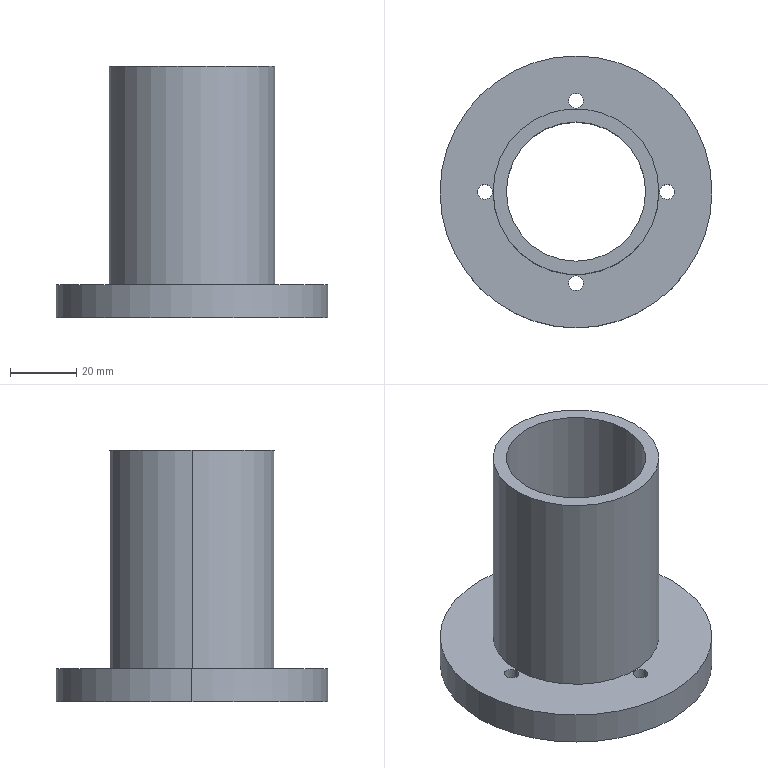Part | SolidWorks | features 3DProfileFeature 1, CirPattern 1, Extrusion 1, HoleWzd 1, ICE 1 | 1 solid | 29 faces | box 82 x 82 x 76 mm | volume 75839 mm3 | cylinder 22 | plane 7 | commonest cylinder face diameters 4.5 x8 8 x8 42 x2 50 x2 82 x2
STEP:
#1=CARTESIAN_POINT('',(31.5,0.,-5.4));
#2=VERTEX_POINT('',#1);
#3=CARTESIAN_POINT('',(23.5,0.,-5.4));
#4=VERTEX_POINT('',#3);
#5=CARTESIAN_POINT('',(27.5,0.,-5.4));
#6=DIRECTION('',(0.,0.,-1.));
#7=DIRECTION('',(-1.,0.,0.));
#8=AXIS2_PLACEMENT_3D('',#5,#6,#7);
#9=CIRCLE('',#8,4.);
#10=EDGE_CURVE('',#2,#4,#9,.T.);
#11=ORIENTED_EDGE('',*,*,#10,.F.);
#12=CARTESIAN_POINT('',(31.5,0.,-10.));
#13=VERTEX_POINT('',#12);
#14=CARTESIAN_POINT('',(31.5,0.,-10.));
#15=DIRECTION('',(0.,0.,-1.));
#16=VECTOR('',#15,1000.);
#17=LINE('',#14,#16);
#18=EDGE_CURVE('',#2,#13,#17,.T.);
#19=ORIENTED_EDGE('',*,*,#18,.T.);
#20=CARTESIAN_POINT('',(23.5,0.,-10.));
#21=VERTEX_POINT('',#20);
#22=CARTESIAN_POINT('',(27.5,0.,-10.));
#23=DIRECTION('',(0.,0.,-1.));
#24=DIRECTION('',(-1.,0.,0.));
#25=AXIS2_PLACEMENT_3D('',#22,#23,#24);
#26=CIRCLE('',#25,4.);
#27=EDGE_CURVE('',#13,#21,#26,.T.);
#28=ORIENTED_EDGE('',*,*,#27,.T.);
#29=CARTESIAN_POINT('',(23.5,0.,-10.));
#30=DIRECTION('',(0.,0.,-1.));
#31=VECTOR('',#30,1000.);
#32=LINE('',#29,#31);
#33=EDGE_CURVE('',#4,#21,#32,.T.);
#34=ORIENTED_EDGE('',*,*,#33,.F.);
#35=EDGE_LOOP('',(#11,#19,#28,#34));
#36=FACE_OUTER_BOUND('',#35,.T.);
#37=CARTESIAN_POINT('',(27.5,0.,-10.));
#38=DIRECTION('',(0.,0.,-1.));
#39=DIRECTION('',(-1.,0.,0.));
#40=AXIS2_PLACEMENT_3D('',#37,#38,#39);
#41=CYLINDRICAL_SURFACE('',#40,4.);
#42=ADVANCED_FACE('',(#36),#41,.F.);
#43=CARTESIAN_POINT('',(29.75,0.,0.));
#44=VERTEX_POINT('',#43);
#45=CARTESIAN_POINT('',(25.25,0.,0.));
#46=VERTEX_POINT('',#45);
#47=CARTESIAN_POINT('',(27.5,0.,0.));
#48=DIRECTION('',(0.,0.,-1.));
#49=DIRECTION('',(-1.,0.,0.));
#50=AXIS2_PLACEMENT_3D('',#47,#48,#49);
#51=CIRCLE('',#50,2.25);
#52=EDGE_CURVE('',#44,#46,#51,.T.);
#53=ORIENTED_EDGE('',*,*,#52,.F.);
#54=CARTESIAN_POINT('',(29.75,0.,-5.4));
#55=VERTEX_POINT('',#54);
#56=CARTESIAN_POINT('',(29.75,0.,-10.));
#57=DIRECTION('',(0.,0.,-1.));
#58=VECTOR('',#57,1000.);
#59=LINE('',#56,#58);
#60=EDGE_CURVE('',#44,#55,#59,.T.);
#61=ORIENTED_EDGE('',*,*,#60,.T.);
#62=CARTESIAN_POINT('',(25.25,0.,-5.4));
#63=VERTEX_POINT('',#62);
#64=CARTESIAN_POINT('',(27.5,0.,-5.4));
#65=DIRECTION('',(0.,0.,-1.));
#66=DIRECTION('',(-1.,0.,0.));
#67=AXIS2_PLACEMENT_3D('',#64,#65,#66);
#68=CIRCLE('',#67,2.25);
#69=EDGE_CURVE('',#55,#63,#68,.T.);
#70=ORIENTED_EDGE('',*,*,#69,.T.);
#71=CARTESIAN_POINT('',(25.25,0.,-10.));
#72=DIRECTION('',(0.,0.,-1.));
#73=VECTOR('',#72,1000.);
#74=LINE('',#71,#73);
#75=EDGE_CURVE('',#46,#63,#74,.T.);
#76=ORIENTED_EDGE('',*,*,#75,.F.);
#77=EDGE_LOOP('',(#53,#61,#70,#76));
#78=FACE_OUTER_BOUND('',#77,.T.);
#79=CARTESIAN_POINT('',(27.5,0.,-10.));
#80=DIRECTION('',(0.,0.,-1.));
#81=DIRECTION('',(-1.,0.,0.));
#82=AXIS2_PLACEMENT_3D('',#79,#80,#81);
#83=CYLINDRICAL_SURFACE('',#82,2.25);
#84=ADVANCED_FACE('',(#78),#83,.F.);
#85=CARTESIAN_POINT('',(4.,27.5,-5.4));
#86=VERTEX_POINT('',#85);
#87=CARTESIAN_POINT('',(-4.,27.5,-5.4));
#88=VERTEX_POINT('',#87);
#89=CARTESIAN_POINT('',(0.,27.5,-5.4));
#90=DIRECTION('',(0.,0.,-1.));
#91=DIRECTION('',(-1.,0.,0.));
#92=AXIS2_PLACEMENT_3D('',#89,#90,#91);
#93=CIRCLE('',#92,4.);
#94=EDGE_CURVE('',#86,#88,#93,.T.);
#95=ORIENTED_EDGE('',*,*,#94,.F.);
#96=CARTESIAN_POINT('',(4.,27.5,-10.));
#97=VERTEX_POINT('',#96);
#98=CARTESIAN_POINT('',(4.,27.5,-10.));
#99=DIRECTION('',(0.,0.,-1.));
#100=VECTOR('',#99,1000.);
#101=LINE('',#98,#100);
#102=EDGE_CURVE('',#86,#97,#101,.T.);
#103=ORIENTED_EDGE('',*,*,#102,.T.);
#104=CARTESIAN_POINT('',(-4.,27.5,-10.));
#105=VERTEX_POINT('',#104);
#106=CARTESIAN_POINT('',(0.,27.5,-10.));
#107=DIRECTION('',(0.,0.,-1.));
#108=DIRECTION('',(-1.,0.,0.));
#109=AXIS2_PLACEMENT_3D('',#106,#107,#108);
#110=CIRCLE('',#109,4.);
#111=EDGE_CURVE('',#97,#105,#110,.T.);
#112=ORIENTED_EDGE('',*,*,#111,.T.);
#113=CARTESIAN_POINT('',(-4.,27.5,-10.));
#114=DIRECTION('',(0.,0.,-1.));
#115=VECTOR('',#114,1000.);
#116=LINE('',#113,#115);
#117=EDGE_CURVE('',#88,#105,#116,.T.);
#118=ORIENTED_EDGE('',*,*,#117,.F.);
#119=EDGE_LOOP('',(#95,#103,#112,#118));
#120=FACE_OUTER_BOUND('',#119,.T.);
#121=CARTESIAN_POINT('',(0.,27.5,-10.));
#122=DIRECTION('',(0.,0.,-1.));
#123=DIRECTION('',(-1.,0.,0.));
#124=AXIS2_PLACEMENT_3D('',#121,#122,#123);
#125=CYLINDRICAL_SURFACE('',#124,4.);
#126=ADVANCED_FACE('',(#120),#125,.F.);
#127=CARTESIAN_POINT('',(2.25,27.5,0.));
#128=VERTEX_POINT('',#127);
#129=CARTESIAN_POINT('',(-2.25,27.5,0.));
#130=VERTEX_POINT('',#129);
#131=CARTESIAN_POINT('',(0.,27.5,0.));
#132=DIRECTION('',(0.,0.,-1.));
#133=DIRECTION('',(-1.,0.,0.));
#134=AXIS2_PLACEMENT_3D('',#131,#132,#133);
#135=CIRCLE('',#134,2.25);
#136=EDGE_CURVE('',#128,#130,#135,.T.);
#137=ORIENTED_EDGE('',*,*,#136,.F.);
#138=CARTESIAN_POINT('',(2.25,27.5,-5.4));
#139=VERTEX_POINT('',#138);
#140=CARTESIAN_POINT('',(2.25,27.5,-10.));
#141=DIRECTION('',(0.,0.,-1.));
#142=VECTOR('',#141,1000.);
#143=LINE('',#140,#142);
#144=EDGE_CURVE('',#128,#139,#143,.T.);
#145=ORIENTED_EDGE('',*,*,#144,.T.);
#146=CARTESIAN_POINT('',(-2.25,27.5,-5.4));
#147=VERTEX_POINT('',#146);
#148=CARTESIAN_POINT('',(0.,27.5,-5.4));
#149=DIRECTION('',(0.,0.,-1.));
#150=DIRECTION('',(-1.,0.,0.));
#151=AXIS2_PLACEMENT_3D('',#148,#149,#150);
#152=CIRCLE('',#151,2.25);
#153=EDGE_CURVE('',#139,#147,#152,.T.);
#154=ORIENTED_EDGE('',*,*,#153,.T.);
#155=CARTESIAN_POINT('',(-2.25,27.5,-10.));
#156=DIRECTION('',(0.,0.,-1.));
#157=VECTOR('',#156,1000.);
#158=LINE('',#155,#157);
#159=EDGE_CURVE('',#130,#147,#158,.T.);
#160=ORIENTED_EDGE('',*,*,#159,.F.);
#161=EDGE_LOOP('',(#137,#145,#154,#160));
#162=FACE_OUTER_BOUND('',#161,.T.);
#163=CARTESIAN_POINT('',(0.,27.5,-10.));
#164=DIRECTION('',(0.,0.,-1.));
#165=DIRECTION('',(-1.,0.,0.));
#166=AXIS2_PLACEMENT_3D('',#163,#164,#165);
#167=CYLINDRICAL_SURFACE('',#166,2.25);
#168=ADVANCED_FACE('',(#162),#167,.F.);
#169=CARTESIAN_POINT('',(-23.5,0.,-5.4));
#170=VERTEX_POINT('',#169);
#171=CARTESIAN_POINT('',(-31.5,0.,-5.4));
#172=VERTEX_POINT('',#171);
#173=CARTESIAN_POINT('',(-27.5,0.,-5.4));
#174=DIRECTION('',(0.,0.,-1.));
#175=DIRECTION('',(-1.,0.,0.));
#176=AXIS2_PLACEMENT_3D('',#173,#174,#175);
#177=CIRCLE('',#176,4.);
#178=EDGE_CURVE('',#170,#172,#177,.T.);
#179=ORIENTED_EDGE('',*,*,#178,.F.);
#180=CARTESIAN_POINT('',(-23.5,0.,-10.));
#181=VERTEX_POINT('',#180);
#182=CARTESIAN_POINT('',(-23.5,0.,-10.));
#183=DIRECTION('',(0.,0.,-1.));
#184=VECTOR('',#183,1000.);
#185=LINE('',#182,#184);
#186=EDGE_CURVE('',#170,#181,#185,.T.);
#187=ORIENTED_EDGE('',*,*,#186,.T.);
#188=CARTESIAN_POINT('',(-31.5,0.,-10.));
#189=VERTEX_POINT('',#188);
#190=CARTESIAN_POINT('',(-27.5,0.,-10.));
#191=DIRECTION('',(0.,0.,-1.));
#192=DIRECTION('',(-1.,0.,0.));
#193=AXIS2_PLACEMENT_3D('',#190,#191,#192);
#194=CIRCLE('',#193,4.);
#195=EDGE_CURVE('',#181,#189,#194,.T.);
#196=ORIENTED_EDGE('',*,*,#195,.T.);
#197=CARTESIAN_POINT('',(-31.5,0.,-10.));
#198=DIRECTION('',(0.,0.,-1.));
#199=VECTOR('',#198,1000.);
#200=LINE('',#197,#199);
#201=EDGE_CURVE('',#172,#189,#200,.T.);
#202=ORIENTED_EDGE('',*,*,#201,.F.);
#203=EDGE_LOOP('',(#179,#187,#196,#202));
#204=FACE_OUTER_BOUND('',#203,.T.);
#205=CARTESIAN_POINT('',(-27.5,0.,-10.));
#206=DIRECTION('',(0.,0.,-1.));
#207=DIRECTION('',(-1.,0.,0.));
#208=AXIS2_PLACEMENT_3D('',#205,#206,#207);
#209=CYLINDRICAL_SURFACE('',#208,4.);
#210=ADVANCED_FACE('',(#204),#209,.F.);
#211=CARTESIAN_POINT('',(-25.25,0.,0.));
#212=VERTEX_POINT('',#211);
#213=CARTESIAN_POINT('',(-29.75,0.,0.));
#214=VERTEX_POINT('',#213);
#215=CARTESIAN_POINT('',(-27.5,0.,0.));
#216=DIRECTION('',(0.,0.,-1.));
#217=DIRECTION('',(-1.,0.,0.));
#218=AXIS2_PLACEMENT_3D('',#215,#216,#217);
#219=CIRCLE('',#218,2.25);
#220=EDGE_CURVE('',#212,#214,#219,.T.);
#221=ORIENTED_EDGE('',*,*,#220,.F.);
#222=CARTESIAN_POINT('',(-25.25,0.,-5.4));
#223=VERTEX_POINT('',#222);
#224=CARTESIAN_POINT('',(-25.25,0.,-10.));
#225=DIRECTION('',(0.,0.,-1.));
#226=VECTOR('',#225,1000.);
#227=LINE('',#224,#226);
#228=EDGE_CURVE('',#212,#223,#227,.T.);
#229=ORIENTED_EDGE('',*,*,#228,.T.);
#230=CARTESIAN_POINT('',(-29.75,0.,-5.4));
#231=VERTEX_POINT('',#230);
#232=CARTESIAN_POINT('',(-27.5,0.,-5.4));
#233=DIRECTION('',(0.,0.,-1.));
#234=DIRECTION('',(-1.,0.,0.));
#235=AXIS2_PLACEMENT_3D('',#232,#233,#234);
#236=CIRCLE('',#235,2.25);
#237=EDGE_CURVE('',#223,#231,#236,.T.);
#238=ORIENTED_EDGE('',*,*,#237,.T.);
#239=CARTESIAN_POINT('',(-29.75,0.,-10.));
#240=DIRECTION('',(0.,0.,-1.));
#241=VECTOR('',#240,1000.);
#242=LINE('',#239,#241);
#243=EDGE_CURVE('',#214,#231,#242,.T.);
#244=ORIENTED_EDGE('',*,*,#243,.F.);
#245=EDGE_LOOP('',(#221,#229,#238,#244));
#246=FACE_OUTER_BOUND('',#245,.T.);
#247=CARTESIAN_POINT('',(-27.5,0.,-10.));
#248=DIRECTION('',(0.,0.,-1.));
#249=DIRECTION('',(-1.,0.,0.));
#250=AXIS2_PLACEMENT_3D('',#247,#248,#249);
#251=CYLINDRICAL_SURFACE('',#250,2.25);
#252=ADVANCED_FACE('',(#246),#251,.F.);
#253=CARTESIAN_POINT('',(4.,-27.5,-5.4));
#254=VERTEX_POINT('',#253);
#255=CARTESIAN_POINT('',(-4.,-27.5,-5.4));
#256=VERTEX_POINT('',#255);
#257=CARTESIAN_POINT('',(0.,-27.5,-5.4));
#258=DIRECTION('',(0.,0.,-1.));
#259=DIRECTION('',(-1.,0.,0.));
#260=AXIS2_PLACEMENT_3D('',#257,#258,#259);
#261=CIRCLE('',#260,4.);
#262=EDGE_CURVE('',#254,#256,#261,.T.);
#263=ORIENTED_EDGE('',*,*,#262,.F.);
#264=CARTESIAN_POINT('',(4.,-27.5,-10.));
#265=VERTEX_POINT('',#264);
#266=CARTESIAN_POINT('',(4.,-27.5,-10.));
#267=DIRECTION('',(0.,0.,-1.));
#268=VECTOR('',#267,1000.);
#269=LINE('',#266,#268);
#270=EDGE_CURVE('',#254,#265,#269,.T.);
#271=ORIENTED_EDGE('',*,*,#270,.T.);
#272=CARTESIAN_POINT('',(-4.,-27.5,-10.));
#273=VERTEX_POINT('',#272);
#274=CARTESIAN_POINT('',(0.,-27.5,-10.));
#275=DIRECTION('',(0.,0.,-1.));
#276=DIRECTION('',(-1.,0.,0.));
#277=AXIS2_PLACEMENT_3D('',#274,#275,#276);
#278=CIRCLE('',#277,4.);
#279=EDGE_CURVE('',#265,#273,#278,.T.);
#280=ORIENTED_EDGE('',*,*,#279,.T.);
#281=CARTESIAN_POINT('',(-4.,-27.5,-10.));
#282=DIRECTION('',(0.,0.,-1.));
#283=VECTOR('',#282,1000.);
#284=LINE('',#281,#283);
#285=EDGE_CURVE('',#256,#273,#284,.T.);
#286=ORIENTED_EDGE('',*,*,#285,.F.);
#287=EDGE_LOOP('',(#263,#271,#280,#286));
#288=FACE_OUTER_BOUND('',#287,.T.);
#289=CARTESIAN_POINT('',(0.,-27.5,-10.));
#290=DIRECTION('',(0.,0.,-1.));
#291=DIRECTION('',(-1.,0.,0.));
#292=AXIS2_PLACEMENT_3D('',#289,#290,#291);
#293=CYLINDRICAL_SURFACE('',#292,4.);
#294=ADVANCED_FACE('',(#288),#293,.F.);
#295=CARTESIAN_POINT('',(2.25,-27.5,0.));
#296=VERTEX_POINT('',#295);
#297=CARTESIAN_POINT('',(-2.25,-27.5,0.));
#298=VERTEX_POINT('',#297);
#299=CARTESIAN_POINT('',(0.,-27.5,0.));
#300=DIRECTION('',(0.,0.,-1.));
#301=DIRECTION('',(-1.,0.,0.));
#302=AXIS2_PLACEMENT_3D('',#299,#300,#301);
#303=CIRCLE('',#302,2.25);
#304=EDGE_CURVE('',#296,#298,#303,.T.);
#305=ORIENTED_EDGE('',*,*,#304,.F.);
#306=CARTESIAN_POINT('',(2.25,-27.5,-5.4));
#307=VERTEX_POINT('',#306);
#308=CARTESIAN_POINT('',(2.25,-27.5,-10.));
#309=DIRECTION('',(0.,0.,-1.));
#310=VECTOR('',#309,1000.);
#311=LINE('',#308,#310);
#312=EDGE_CURVE('',#296,#307,#311,.T.);
#313=ORIENTED_EDGE('',*,*,#312,.T.);
#314=CARTESIAN_POINT('',(-2.25,-27.5,-5.4));
#315=VERTEX_POINT('',#314);
#316=CARTESIAN_POINT('',(0.,-27.5,-5.4));
#317=DIRECTION('',(0.,0.,-1.));
#318=DIRECTION('',(-1.,0.,0.));
#319=AXIS2_PLACEMENT_3D('',#316,#317,#318);
#320=CIRCLE('',#319,2.25);
#321=EDGE_CURVE('',#307,#315,#320,.T.);
#322=ORIENTED_EDGE('',*,*,#321,.T.);
#323=CARTESIAN_POINT('',(-2.25,-27.5,-10.));
#324=DIRECTION('',(0.,0.,-1.));
#325=VECTOR('',#324,1000.);
#326=LINE('',#323,#325);
#327=EDGE_CURVE('',#298,#315,#326,.T.);
#328=ORIENTED_EDGE('',*,*,#327,.F.);
#329=EDGE_LOOP('',(#305,#313,#322,#328));
#330=FACE_OUTER_BOUND('',#329,.T.);
#331=CARTESIAN_POINT('',(0.,-27.5,-10.));
#332=DIRECTION('',(0.,0.,-1.));
#333=DIRECTION('',(-1.,0.,0.));
#334=AXIS2_PLACEMENT_3D('',#331,#332,#333);
#335=CYLINDRICAL_SURFACE('',#334,2.25);
#336=ADVANCED_FACE('',(#330),#335,.F.);
#337=CARTESIAN_POINT('',(-41.,0.,-10.));
#338=VERTEX_POINT('',#337);
#339=CARTESIAN_POINT('',(41.,0.,-10.));
#340=VERTEX_POINT('',#339);
#341=CARTESIAN_POINT('',(0.,0.,-10.));
#342=DIRECTION('',(0.,0.,-1.));
#343=DIRECTION('',(-1.,0.,0.));
#344=AXIS2_PLACEMENT_3D('',#341,#342,#343);
#345=CIRCLE('',#344,41.);
#346=EDGE_CURVE('',#338,#340,#345,.T.);
#347=ORIENTED_EDGE('',*,*,#346,.F.);
#348=CARTESIAN_POINT('',(-41.,0.,0.));
#349=VERTEX_POINT('',#348);
#350=CARTESIAN_POINT('',(-41.,0.,-10.));
#351=DIRECTION('',(0.,0.,1.));
#352=VECTOR('',#351,1000.);
#353=LINE('',#350,#352);
#354=EDGE_CURVE('',#338,#349,#353,.T.);
#355=ORIENTED_EDGE('',*,*,#354,.T.);
#356=CARTESIAN_POINT('',(41.,0.,0.));
#357=VERTEX_POINT('',#356);
#358=CARTESIAN_POINT('',(0.,0.,0.));
#359=DIRECTION('',(0.,0.,-1.));
#360=DIRECTION('',(-1.,0.,0.));
#361=AXIS2_PLACEMENT_3D('',#358,#359,#360);
#362=CIRCLE('',#361,41.);
#363=EDGE_CURVE('',#349,#357,#362,.T.);
#364=ORIENTED_EDGE('',*,*,#363,.T.);
#365=CARTESIAN_POINT('',(41.,0.,-10.));
#366=DIRECTION('',(0.,0.,1.));
#367=VECTOR('',#366,1000.);
#368=LINE('',#365,#367);
#369=EDGE_CURVE('',#340,#357,#368,.T.);
#370=ORIENTED_EDGE('',*,*,#369,.F.);
#371=EDGE_LOOP('',(#347,#355,#364,#370));
#372=FACE_OUTER_BOUND('',#371,.T.);
#373=CARTESIAN_POINT('',(0.,0.,-10.));
#374=DIRECTION('',(0.,0.,1.));
#375=DIRECTION('',(1.,0.,0.));
#376=AXIS2_PLACEMENT_3D('',#373,#374,#375);
#377=CYLINDRICAL_SURFACE('',#376,41.);
#378=ADVANCED_FACE('',(#372),#377,.T.);
#379=CARTESIAN_POINT('',(-21.,0.,66.));
#380=VERTEX_POINT('',#379);
#381=CARTESIAN_POINT('',(21.,0.,66.));
#382=VERTEX_POINT('',#381);
#383=CARTESIAN_POINT('',(0.,0.,66.));
#384=DIRECTION('',(0.,0.,1.));
#385=DIRECTION('',(1.,0.,0.));
#386=AXIS2_PLACEMENT_3D('',#383,#384,#385);
#387=CIRCLE('',#386,21.);
#388=EDGE_CURVE('',#380,#382,#387,.T.);
#389=ORIENTED_EDGE('',*,*,#388,.T.);
#390=CARTESIAN_POINT('',(21.,0.,-10.));
#391=VERTEX_POINT('',#390);
#392=CARTESIAN_POINT('',(21.,0.,66.));
#393=DIRECTION('',(0.,0.,-1.));
#394=VECTOR('',#393,1000.);
#395=LINE('',#392,#394);
#396=EDGE_CURVE('',#382,#391,#395,.T.);
#397=ORIENTED_EDGE('',*,*,#396,.T.);
#398=CARTESIAN_POINT('',(-21.,0.,-10.));
#399=VERTEX_POINT('',#398);
#400=CARTESIAN_POINT('',(0.,0.,-10.));
#401=DIRECTION('',(0.,0.,-1.));
#402=DIRECTION('',(-1.,0.,0.));
#403=AXIS2_PLACEMENT_3D('',#400,#401,#402);
#404=CIRCLE('',#403,21.);
#405=EDGE_CURVE('',#391,#399,#404,.T.);
#406=ORIENTED_EDGE('',*,*,#405,.T.);
#407=CARTESIAN_POINT('',(-21.,0.,66.));
#408=DIRECTION('',(0.,0.,-1.));
#409=VECTOR('',#408,1000.);
#410=LINE('',#407,#409);
#411=EDGE_CURVE('',#380,#399,#410,.T.);
#412=ORIENTED_EDGE('',*,*,#411,.F.);
#413=EDGE_LOOP('',(#389,#397,#406,#412));
#414=FACE_OUTER_BOUND('',#413,.T.);
#415=CARTESIAN_POINT('',(0.,0.,66.));
#416=DIRECTION('',(0.,0.,-1.));
#417=DIRECTION('',(-1.,0.,0.));
#418=AXIS2_PLACEMENT_3D('',#415,#416,#417);
#419=CYLINDRICAL_SURFACE('',#418,21.);
#420=ADVANCED_FACE('',(#414),#419,.F.);
#421=CARTESIAN_POINT('',(25.,0.,66.));
#422=VERTEX_POINT('',#421);
#423=CARTESIAN_POINT('',(-25.,0.,66.));
#424=VERTEX_POINT('',#423);
#425=CARTESIAN_POINT('',(0.,0.,66.));
#426=DIRECTION('',(0.,0.,1.));
#427=DIRECTION('',(1.,0.,0.));
#428=AXIS2_PLACEMENT_3D('',#425,#426,#427);
#429=CIRCLE('',#428,25.);
#430=EDGE_CURVE('',#422,#424,#429,.T.);
#431=ORIENTED_EDGE('',*,*,#430,.F.);
#432=CARTESIAN_POINT('',(25.,0.,0.));
#433=VERTEX_POINT('',#432);
#434=CARTESIAN_POINT('',(25.,0.,66.));
#435=DIRECTION('',(0.,0.,-1.));
#436=VECTOR('',#435,1000.);
#437=LINE('',#434,#436);
#438=EDGE_CURVE('',#422,#433,#437,.T.);
#439=ORIENTED_EDGE('',*,*,#438,.T.);
#440=CARTESIAN_POINT('',(-25.,0.,0.));
#441=VERTEX_POINT('',#440);
#442=CARTESIAN_POINT('',(0.,0.,0.));
#443=DIRECTION('',(0.,0.,1.));
#444=DIRECTION('',(1.,0.,0.));
#445=AXIS2_PLACEMENT_3D('',#442,#443,#444);
#446=CIRCLE('',#445,25.);
#447=EDGE_CURVE('',#433,#441,#446,.T.);
#448=ORIENTED_EDGE('',*,*,#447,.T.);
#449=CARTESIAN_POINT('',(-25.,0.,66.));
#450=DIRECTION('',(0.,0.,-1.));
#451=VECTOR('',#450,1000.);
#452=LINE('',#449,#451);
#453=EDGE_CURVE('',#424,#441,#452,.T.);
#454=ORIENTED_EDGE('',*,*,#453,.F.);
#455=EDGE_LOOP('',(#431,#439,#448,#454));
#456=FACE_OUTER_BOUND('',#455,.T.);
#457=CARTESIAN_POINT('',(0.,0.,66.));
#458=DIRECTION('',(0.,0.,-1.));
#459=DIRECTION('',(-1.,0.,0.));
#460=AXIS2_PLACEMENT_3D('',#457,#458,#459);
#461=CYLINDRICAL_SURFACE('',#460,25.);
#462=ADVANCED_FACE('',(#456),#461,.T.);
#463=CARTESIAN_POINT('',(0.,0.,66.));
#464=DIRECTION('',(0.,0.,1.));
#465=DIRECTION('',(1.,0.,0.));
#466=AXIS2_PLACEMENT_3D('',#463,#464,#465);
#467=CIRCLE('',#466,25.);
#468=EDGE_CURVE('',#424,#422,#467,.T.);
#469=ORIENTED_EDGE('',*,*,#468,.T.);
#470=ORIENTED_EDGE('',*,*,#430,.T.);
#471=EDGE_LOOP('',(#469,#470));
#472=FACE_OUTER_BOUND('',#471,.T.);
#473=ORIENTED_EDGE('',*,*,#388,.F.);
#474=CARTESIAN_POINT('',(0.,0.,66.));
#475=DIRECTION('',(0.,0.,1.));
#476=DIRECTION('',(1.,0.,0.));
#477=AXIS2_PLACEMENT_3D('',#474,#475,#476);
#478=CIRCLE('',#477,21.);
#479=EDGE_CURVE('',#382,#380,#478,.T.);
#480=ORIENTED_EDGE('',*,*,#479,.F.);
#481=EDGE_LOOP('',(#473,#480));
#482=FACE_BOUND('',#481,.T.);
#483=CARTESIAN_POINT('',(0.,0.,66.));
#484=DIRECTION('',(0.,0.,1.));
#485=DIRECTION('',(1.,0.,0.));
#486=AXIS2_PLACEMENT_3D('',#483,#484,#485);
#487=PLANE('',#486);
#488=ADVANCED_FACE('',(#472,#482),#487,.T.);
#489=ORIENTED_EDGE('',*,*,#438,.F.);
#490=ORIENTED_EDGE('',*,*,#468,.F.);
#491=ORIENTED_EDGE('',*,*,#453,.T.);
#492=CARTESIAN_POINT('',(0.,0.,0.));
#493=DIRECTION('',(0.,0.,1.));
#494=DIRECTION('',(1.,0.,0.));
#495=AXIS2_PLACEMENT_3D('',#492,#493,#494);
#496=CIRCLE('',#495,25.);
#497=EDGE_CURVE('',#441,#433,#496,.T.);
#498=ORIENTED_EDGE('',*,*,#497,.T.);
#499=EDGE_LOOP('',(#489,#490,#491,#498));
#500=FACE_OUTER_BOUND('',#499,.T.);
#501=CARTESIAN_POINT('',(0.,0.,66.));
#502=DIRECTION('',(0.,0.,-1.));
#503=DIRECTION('',(-1.,0.,0.));
#504=AXIS2_PLACEMENT_3D('',#501,#502,#503);
#505=CYLINDRICAL_SURFACE('',#504,25.);
#506=ADVANCED_FACE('',(#500),#505,.T.);
#507=ORIENTED_EDGE('',*,*,#396,.F.);
#508=ORIENTED_EDGE('',*,*,#479,.T.);
#509=ORIENTED_EDGE('',*,*,#411,.T.);
#510=CARTESIAN_POINT('',(0.,0.,-10.));
#511=DIRECTION('',(0.,0.,-1.));
#512=DIRECTION('',(-1.,0.,0.));
#513=AXIS2_PLACEMENT_3D('',#510,#511,#512);
#514=CIRCLE('',#513,21.);
#515=EDGE_CURVE('',#399,#391,#514,.T.);
#516=ORIENTED_EDGE('',*,*,#515,.T.);
#517=EDGE_LOOP('',(#507,#508,#509,#516));
#518=FACE_OUTER_BOUND('',#517,.T.);
#519=CARTESIAN_POINT('',(0.,0.,66.));
#520=DIRECTION('',(0.,0.,-1.));
#521=DIRECTION('',(-1.,0.,0.));
#522=AXIS2_PLACEMENT_3D('',#519,#520,#521);
#523=CYLINDRICAL_SURFACE('',#522,21.);
#524=ADVANCED_FACE('',(#518),#523,.F.);
#525=CARTESIAN_POINT('',(27.5,0.,-10.));
#526=DIRECTION('',(0.,0.,-1.));
#527=DIRECTION('',(-1.,0.,0.));
#528=AXIS2_PLACEMENT_3D('',#525,#526,#527);
#529=CIRCLE('',#528,4.);
#530=EDGE_CURVE('',#21,#13,#529,.T.);
#531=ORIENTED_EDGE('',*,*,#530,.F.);
#532=ORIENTED_EDGE('',*,*,#27,.F.);
#533=EDGE_LOOP('',(#531,#532));
#534=FACE_BOUND('',#533,.T.);
#535=CARTESIAN_POINT('',(0.,27.5,-10.));
#536=DIRECTION('',(0.,0.,-1.));
#537=DIRECTION('',(-1.,0.,0.));
#538=AXIS2_PLACEMENT_3D('',#535,#536,#537);
#539=CIRCLE('',#538,4.);
#540=EDGE_CURVE('',#105,#97,#539,.T.);
#541=ORIENTED_EDGE('',*,*,#540,.F.);
#542=ORIENTED_EDGE('',*,*,#111,.F.);
#543=EDGE_LOOP('',(#541,#542));
#544=FACE_BOUND('',#543,.T.);
#545=CARTESIAN_POINT('',(-27.5,0.,-10.));
#546=DIRECTION('',(0.,0.,-1.));
#547=DIRECTION('',(-1.,0.,0.));
#548=AXIS2_PLACEMENT_3D('',#545,#546,#547);
#549=CIRCLE('',#548,4.);
#550=EDGE_CURVE('',#189,#181,#549,.T.);
#551=ORIENTED_EDGE('',*,*,#550,.F.);
#552=ORIENTED_EDGE('',*,*,#195,.F.);
#553=EDGE_LOOP('',(#551,#552));
#554=FACE_BOUND('',#553,.T.);
#555=CARTESIAN_POINT('',(0.,-27.5,-10.));
#556=DIRECTION('',(0.,0.,-1.));
#557=DIRECTION('',(-1.,0.,0.));
#558=AXIS2_PLACEMENT_3D('',#555,#556,#557);
#559=CIRCLE('',#558,4.);
#560=EDGE_CURVE('',#273,#265,#559,.T.);
#561=ORIENTED_EDGE('',*,*,#560,.F.);
#562=ORIENTED_EDGE('',*,*,#279,.F.);
#563=EDGE_LOOP('',(#561,#562));
#564=FACE_BOUND('',#563,.T.);
#565=CARTESIAN_POINT('',(0.,0.,-10.));
#566=DIRECTION('',(0.,0.,-1.));
#567=DIRECTION('',(-1.,0.,0.));
#568=AXIS2_PLACEMENT_3D('',#565,#566,#567);
#569=CIRCLE('',#568,41.);
#570=EDGE_CURVE('',#340,#338,#569,.T.);
#571=ORIENTED_EDGE('',*,*,#570,.T.);
#572=ORIENTED_EDGE('',*,*,#346,.T.);
#573=EDGE_LOOP('',(#571,#572));
#574=FACE_OUTER_BOUND('',#573,.T.);
#575=ORIENTED_EDGE('',*,*,#515,.F.);
#576=ORIENTED_EDGE('',*,*,#405,.F.);
#577=EDGE_LOOP('',(#575,#576));
#578=FACE_BOUND('',#577,.T.);
#579=CARTESIAN_POINT('',(0.,0.,-10.));
#580=DIRECTION('',(0.,0.,-1.));
#581=DIRECTION('',(-1.,0.,0.));
#582=AXIS2_PLACEMENT_3D('',#579,#580,#581);
#583=PLANE('',#582);
#584=ADVANCED_FACE('',(#534,#544,#554,#564,#574,#578),#583,.T.);
#585=CARTESIAN_POINT('',(27.5,0.,0.));
#586=DIRECTION('',(0.,0.,-1.));
#587=DIRECTION('',(-1.,0.,0.));
#588=AXIS2_PLACEMENT_3D('',#585,#586,#587);
#589=CIRCLE('',#588,2.25);
#590=EDGE_CURVE('',#46,#44,#589,.T.);
#591=ORIENTED_EDGE('',*,*,#590,.T.);
#592=ORIENTED_EDGE('',*,*,#52,.T.);
#593=EDGE_LOOP('',(#591,#592));
#594=FACE_BOUND('',#593,.T.);
#595=CARTESIAN_POINT('',(0.,27.5,0.));
#596=DIRECTION('',(0.,0.,-1.));
#597=DIRECTION('',(-1.,0.,0.));
#598=AXIS2_PLACEMENT_3D('',#595,#596,#597);
#599=CIRCLE('',#598,2.25);
#600=EDGE_CURVE('',#130,#128,#599,.T.);
#601=ORIENTED_EDGE('',*,*,#600,.T.);
#602=ORIENTED_EDGE('',*,*,#136,.T.);
#603=EDGE_LOOP('',(#601,#602));
#604=FACE_BOUND('',#603,.T.);
#605=CARTESIAN_POINT('',(-27.5,0.,0.));
#606=DIRECTION('',(0.,0.,-1.));
#607=DIRECTION('',(-1.,0.,0.));
#608=AXIS2_PLACEMENT_3D('',#605,#606,#607);
#609=CIRCLE('',#608,2.25);
#610=EDGE_CURVE('',#214,#212,#609,.T.);
#611=ORIENTED_EDGE('',*,*,#610,.T.);
#612=ORIENTED_EDGE('',*,*,#220,.T.);
#613=EDGE_LOOP('',(#611,#612));
#614=FACE_BOUND('',#613,.T.);
#615=CARTESIAN_POINT('',(0.,-27.5,0.));
#616=DIRECTION('',(0.,0.,-1.));
#617=DIRECTION('',(-1.,0.,0.));
#618=AXIS2_PLACEMENT_3D('',#615,#616,#617);
#619=CIRCLE('',#618,2.25);
#620=EDGE_CURVE('',#298,#296,#619,.T.);
#621=ORIENTED_EDGE('',*,*,#620,.T.);
#622=ORIENTED_EDGE('',*,*,#304,.T.);
#623=EDGE_LOOP('',(#621,#622));
#624=FACE_BOUND('',#623,.T.);
#625=ORIENTED_EDGE('',*,*,#497,.F.);
#626=ORIENTED_EDGE('',*,*,#447,.F.);
#627=EDGE_LOOP('',(#625,#626));
#628=FACE_BOUND('',#627,.T.);
#629=CARTESIAN_POINT('',(0.,0.,0.));
#630=DIRECTION('',(0.,0.,-1.));
#631=DIRECTION('',(-1.,0.,0.));
#632=AXIS2_PLACEMENT_3D('',#629,#630,#631);
#633=CIRCLE('',#632,41.);
#634=EDGE_CURVE('',#357,#349,#633,.T.);
#635=ORIENTED_EDGE('',*,*,#634,.F.);
#636=ORIENTED_EDGE('',*,*,#363,.F.);
#637=EDGE_LOOP('',(#635,#636));
#638=FACE_OUTER_BOUND('',#637,.T.);
#639=CARTESIAN_POINT('',(0.,0.,0.));
#640=DIRECTION('',(0.,0.,-1.));
#641=DIRECTION('',(-1.,0.,0.));
#642=AXIS2_PLACEMENT_3D('',#639,#640,#641);
#643=PLANE('',#642);
#644=ADVANCED_FACE('',(#594,#604,#614,#624,#628,#638),#643,.F.);
#645=ORIENTED_EDGE('',*,*,#354,.F.);
#646=ORIENTED_EDGE('',*,*,#570,.F.);
#647=ORIENTED_EDGE('',*,*,#369,.T.);
#648=ORIENTED_EDGE('',*,*,#634,.T.);
#649=EDGE_LOOP('',(#645,#646,#647,#648));
#650=FACE_OUTER_BOUND('',#649,.T.);
#651=CARTESIAN_POINT('',(0.,0.,-10.));
#652=DIRECTION('',(0.,0.,1.));
#653=DIRECTION('',(1.,0.,0.));
#654=AXIS2_PLACEMENT_3D('',#651,#652,#653);
#655=CYLINDRICAL_SURFACE('',#654,41.);
#656=ADVANCED_FACE('',(#650),#655,.T.);
#657=ORIENTED_EDGE('',*,*,#312,.F.);
#658=ORIENTED_EDGE('',*,*,#620,.F.);
#659=ORIENTED_EDGE('',*,*,#327,.T.);
#660=CARTESIAN_POINT('',(0.,-27.5,-5.4));
#661=DIRECTION('',(0.,0.,-1.));
#662=DIRECTION('',(-1.,0.,0.));
#663=AXIS2_PLACEMENT_3D('',#660,#661,#662);
#664=CIRCLE('',#663,2.25);
#665=EDGE_CURVE('',#315,#307,#664,.T.);
#666=ORIENTED_EDGE('',*,*,#665,.T.);
#667=EDGE_LOOP('',(#657,#658,#659,#666));
#668=FACE_OUTER_BOUND('',#667,.T.);
#669=CARTESIAN_POINT('',(0.,-27.5,-10.));
#670=DIRECTION('',(0.,0.,-1.));
#671=DIRECTION('',(-1.,0.,0.));
#672=AXIS2_PLACEMENT_3D('',#669,#670,#671);
#673=CYLINDRICAL_SURFACE('',#672,2.25);
#674=ADVANCED_FACE('',(#668),#673,.F.);
#675=ORIENTED_EDGE('',*,*,#665,.F.);
#676=ORIENTED_EDGE('',*,*,#321,.F.);
#677=EDGE_LOOP('',(#675,#676));
#678=FACE_BOUND('',#677,.T.);
#679=CARTESIAN_POINT('',(0.,-27.5,-5.4));
#680=DIRECTION('',(0.,0.,-1.));
#681=DIRECTION('',(-1.,0.,0.));
#682=AXIS2_PLACEMENT_3D('',#679,#680,#681);
#683=CIRCLE('',#682,4.);
#684=EDGE_CURVE('',#256,#254,#683,.T.);
#685=ORIENTED_EDGE('',*,*,#684,.T.);
#686=ORIENTED_EDGE('',*,*,#262,.T.);
#687=EDGE_LOOP('',(#685,#686));
#688=FACE_OUTER_BOUND('',#687,.T.);
#689=CARTESIAN_POINT('',(2.25,-27.5,-5.4));
#690=DIRECTION('',(0.,0.,1.));
#691=DIRECTION('',(1.,0.,0.));
#692=AXIS2_PLACEMENT_3D('',#689,#690,#691);
#693=PLANE('',#692);
#694=ADVANCED_FACE('',(#678,#688),#693,.F.);
#695=ORIENTED_EDGE('',*,*,#270,.F.);
#696=ORIENTED_EDGE('',*,*,#684,.F.);
#697=ORIENTED_EDGE('',*,*,#285,.T.);
#698=ORIENTED_EDGE('',*,*,#560,.T.);
#699=EDGE_LOOP('',(#695,#696,#697,#698));
#700=FACE_OUTER_BOUND('',#699,.T.);
#701=CARTESIAN_POINT('',(0.,-27.5,-10.));
#702=DIRECTION('',(0.,0.,-1.));
#703=DIRECTION('',(-1.,0.,0.));
#704=AXIS2_PLACEMENT_3D('',#701,#702,#703);
#705=CYLINDRICAL_SURFACE('',#704,4.);
#706=ADVANCED_FACE('',(#700),#705,.F.);
#707=ORIENTED_EDGE('',*,*,#228,.F.);
#708=ORIENTED_EDGE('',*,*,#610,.F.);
#709=ORIENTED_EDGE('',*,*,#243,.T.);
#710=CARTESIAN_POINT('',(-27.5,0.,-5.4));
#711=DIRECTION('',(0.,0.,-1.));
#712=DIRECTION('',(-1.,0.,0.));
#713=AXIS2_PLACEMENT_3D('',#710,#711,#712);
#714=CIRCLE('',#713,2.25);
#715=EDGE_CURVE('',#231,#223,#714,.T.);
#716=ORIENTED_EDGE('',*,*,#715,.T.);
#717=EDGE_LOOP('',(#707,#708,#709,#716));
#718=FACE_OUTER_BOUND('',#717,.T.);
#719=CARTESIAN_POINT('',(-27.5,0.,-10.));
#720=DIRECTION('',(0.,0.,-1.));
#721=DIRECTION('',(-1.,0.,0.));
#722=AXIS2_PLACEMENT_3D('',#719,#720,#721);
#723=CYLINDRICAL_SURFACE('',#722,2.25);
#724=ADVANCED_FACE('',(#718),#723,.F.);
#725=ORIENTED_EDGE('',*,*,#715,.F.);
#726=ORIENTED_EDGE('',*,*,#237,.F.);
#727=EDGE_LOOP('',(#725,#726));
#728=FACE_BOUND('',#727,.T.);
#729=CARTESIAN_POINT('',(-27.5,0.,-5.4));
#730=DIRECTION('',(0.,0.,-1.));
#731=DIRECTION('',(-1.,0.,0.));
#732=AXIS2_PLACEMENT_3D('',#729,#730,#731);
#733=CIRCLE('',#732,4.);
#734=EDGE_CURVE('',#172,#170,#733,.T.);
#735=ORIENTED_EDGE('',*,*,#734,.T.);
#736=ORIENTED_EDGE('',*,*,#178,.T.);
#737=EDGE_LOOP('',(#735,#736));
#738=FACE_OUTER_BOUND('',#737,.T.);
#739=CARTESIAN_POINT('',(-25.25,0.,-5.4));
#740=DIRECTION('',(0.,0.,1.));
#741=DIRECTION('',(1.,0.,0.));
#742=AXIS2_PLACEMENT_3D('',#739,#740,#741);
#743=PLANE('',#742);
#744=ADVANCED_FACE('',(#728,#738),#743,.F.);
#745=ORIENTED_EDGE('',*,*,#186,.F.);
#746=ORIENTED_EDGE('',*,*,#734,.F.);
#747=ORIENTED_EDGE('',*,*,#201,.T.);
#748=ORIENTED_EDGE('',*,*,#550,.T.);
#749=EDGE_LOOP('',(#745,#746,#747,#748));
#750=FACE_OUTER_BOUND('',#749,.T.);
#751=CARTESIAN_POINT('',(-27.5,0.,-10.));
#752=DIRECTION('',(0.,0.,-1.));
#753=DIRECTION('',(-1.,0.,0.));
#754=AXIS2_PLACEMENT_3D('',#751,#752,#753);
#755=CYLINDRICAL_SURFACE('',#754,4.);
#756=ADVANCED_FACE('',(#750),#755,.F.);
#757=ORIENTED_EDGE('',*,*,#144,.F.);
#758=ORIENTED_EDGE('',*,*,#600,.F.);
#759=ORIENTED_EDGE('',*,*,#159,.T.);
#760=CARTESIAN_POINT('',(0.,27.5,-5.4));
#761=DIRECTION('',(0.,0.,-1.));
#762=DIRECTION('',(-1.,0.,0.));
#763=AXIS2_PLACEMENT_3D('',#760,#761,#762);
#764=CIRCLE('',#763,2.25);
#765=EDGE_CURVE('',#147,#139,#764,.T.);
#766=ORIENTED_EDGE('',*,*,#765,.T.);
#767=EDGE_LOOP('',(#757,#758,#759,#766));
#768=FACE_OUTER_BOUND('',#767,.T.);
#769=CARTESIAN_POINT('',(0.,27.5,-10.));
#770=DIRECTION('',(0.,0.,-1.));
#771=DIRECTION('',(-1.,0.,0.));
#772=AXIS2_PLACEMENT_3D('',#769,#770,#771);
#773=CYLINDRICAL_SURFACE('',#772,2.25);
#774=ADVANCED_FACE('',(#768),#773,.F.);
#775=ORIENTED_EDGE('',*,*,#765,.F.);
#776=ORIENTED_EDGE('',*,*,#153,.F.);
#777=EDGE_LOOP('',(#775,#776));
#778=FACE_BOUND('',#777,.T.);
#779=CARTESIAN_POINT('',(0.,27.5,-5.4));
#780=DIRECTION('',(0.,0.,-1.));
#781=DIRECTION('',(-1.,0.,0.));
#782=AXIS2_PLACEMENT_3D('',#779,#780,#781);
#783=CIRCLE('',#782,4.);
#784=EDGE_CURVE('',#88,#86,#783,.T.);
#785=ORIENTED_EDGE('',*,*,#784,.T.);
#786=ORIENTED_EDGE('',*,*,#94,.T.);
#787=EDGE_LOOP('',(#785,#786));
#788=FACE_OUTER_BOUND('',#787,.T.);
#789=CARTESIAN_POINT('',(2.25,27.5,-5.4));
#790=DIRECTION('',(0.,0.,1.));
#791=DIRECTION('',(1.,0.,0.));
#792=AXIS2_PLACEMENT_3D('',#789,#790,#791);
#793=PLANE('',#792);
#794=ADVANCED_FACE('',(#778,#788),#793,.F.);
#795=ORIENTED_EDGE('',*,*,#102,.F.);
#796=ORIENTED_EDGE('',*,*,#784,.F.);
#797=ORIENTED_EDGE('',*,*,#117,.T.);
#798=ORIENTED_EDGE('',*,*,#540,.T.);
#799=EDGE_LOOP('',(#795,#796,#797,#798));
#800=FACE_OUTER_BOUND('',#799,.T.);
#801=CARTESIAN_POINT('',(0.,27.5,-10.));
#802=DIRECTION('',(0.,0.,-1.));
#803=DIRECTION('',(-1.,0.,0.));
#804=AXIS2_PLACEMENT_3D('',#801,#802,#803);
#805=CYLINDRICAL_SURFACE('',#804,4.);
#806=ADVANCED_FACE('',(#800),#805,.F.);
#807=ORIENTED_EDGE('',*,*,#60,.F.);
#808=ORIENTED_EDGE('',*,*,#590,.F.);
#809=ORIENTED_EDGE('',*,*,#75,.T.);
#810=CARTESIAN_POINT('',(27.5,0.,-5.4));
#811=DIRECTION('',(0.,0.,-1.));
#812=DIRECTION('',(-1.,0.,0.));
#813=AXIS2_PLACEMENT_3D('',#810,#811,#812);
#814=CIRCLE('',#813,2.25);
#815=EDGE_CURVE('',#63,#55,#814,.T.);
#816=ORIENTED_EDGE('',*,*,#815,.T.);
#817=EDGE_LOOP('',(#807,#808,#809,#816));
#818=FACE_OUTER_BOUND('',#817,.T.);
#819=CARTESIAN_POINT('',(27.5,0.,-10.));
#820=DIRECTION('',(0.,0.,-1.));
#821=DIRECTION('',(-1.,0.,0.));
#822=AXIS2_PLACEMENT_3D('',#819,#820,#821);
#823=CYLINDRICAL_SURFACE('',#822,2.25);
#824=ADVANCED_FACE('',(#818),#823,.F.);
#825=ORIENTED_EDGE('',*,*,#815,.F.);
#826=ORIENTED_EDGE('',*,*,#69,.F.);
#827=EDGE_LOOP('',(#825,#826));
#828=FACE_BOUND('',#827,.T.);
#829=CARTESIAN_POINT('',(27.5,0.,-5.4));
#830=DIRECTION('',(0.,0.,-1.));
#831=DIRECTION('',(-1.,0.,0.));
#832=AXIS2_PLACEMENT_3D('',#829,#830,#831);
#833=CIRCLE('',#832,4.);
#834=EDGE_CURVE('',#4,#2,#833,.T.);
#835=ORIENTED_EDGE('',*,*,#834,.T.);
#836=ORIENTED_EDGE('',*,*,#10,.T.);
#837=EDGE_LOOP('',(#835,#836));
#838=FACE_OUTER_BOUND('',#837,.T.);
#839=CARTESIAN_POINT('',(29.75,0.,-5.4));
#840=DIRECTION('',(0.,0.,1.));
#841=DIRECTION('',(1.,0.,0.));
#842=AXIS2_PLACEMENT_3D('',#839,#840,#841);
#843=PLANE('',#842);
#844=ADVANCED_FACE('',(#828,#838),#843,.F.);
#845=ORIENTED_EDGE('',*,*,#18,.F.);
#846=ORIENTED_EDGE('',*,*,#834,.F.);
#847=ORIENTED_EDGE('',*,*,#33,.T.);
#848=ORIENTED_EDGE('',*,*,#530,.T.);
#849=EDGE_LOOP('',(#845,#846,#847,#848));
#850=FACE_OUTER_BOUND('',#849,.T.);
#851=CARTESIAN_POINT('',(27.5,0.,-10.));
#852=DIRECTION('',(0.,0.,-1.));
#853=DIRECTION('',(-1.,0.,0.));
#854=AXIS2_PLACEMENT_3D('',#851,#852,#853);
#855=CYLINDRICAL_SURFACE('',#854,4.);
#856=ADVANCED_FACE('',(#850),#855,.F.);
#857=CLOSED_SHELL('',(#42,#84,#126,#168,#210,#252,#294,#336,#378,#420,#462,#488,#506,#524,#584,#644,#656,#674,#694,#706,#724,#744,#756,#774,#794,#806,#824,#844,#856));
#858=MANIFOLD_SOLID_BREP('',#857);
#859=CARTESIAN_POINT('',(0.,0.,0.));
#860=DIRECTION('',(0.,0.,1.));
#861=DIRECTION('',(1.,0.,0.));
#862=AXIS2_PLACEMENT_3D('',#859,#860,#861);
#863=(LENGTH_UNIT()NAMED_UNIT(*)SI_UNIT(.MILLI.,.METRE.));
#864=UNCERTAINTY_MEASURE_WITH_UNIT(LENGTH_MEASURE(0.00001),#863,'','');
#865=(NAMED_UNIT(*)PLANE_ANGLE_UNIT()SI_UNIT($,.RADIAN.));
#866=(NAMED_UNIT(*)SI_UNIT($,.STERADIAN.)SOLID_ANGLE_UNIT());
#867=(GEOMETRIC_REPRESENTATION_CONTEXT(3)GLOBAL_UNCERTAINTY_ASSIGNED_CONTEXT((#864))GLOBAL_UNIT_ASSIGNED_CONTEXT((#863,#865,#866))REPRESENTATION_CONTEXT('',''));
#868=ADVANCED_BREP_SHAPE_REPRESENTATION('',(#858,#862),#867);